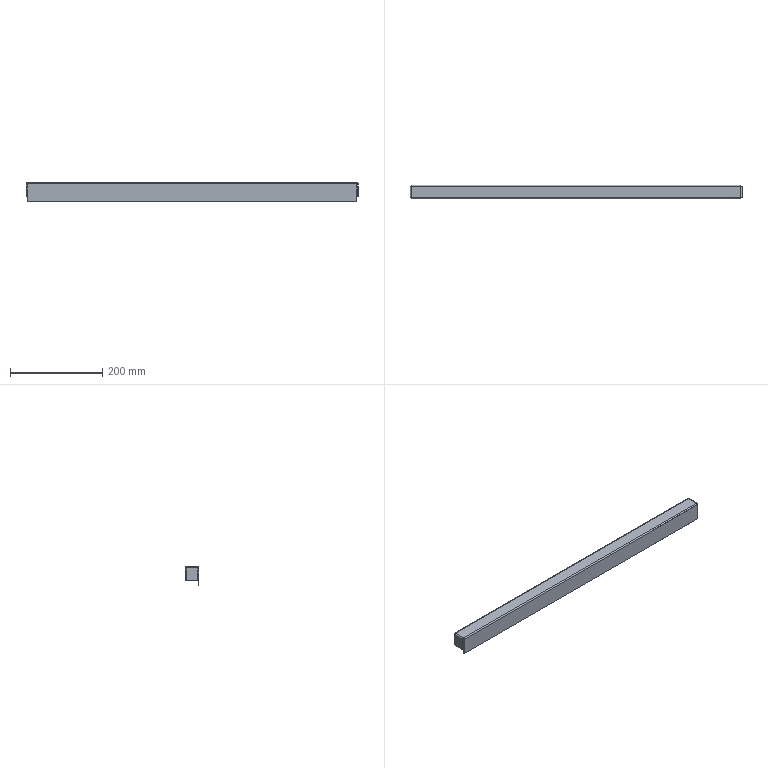Part | STEP file | Front sheet metal baffle | 1 solid | 46 faces | box 720 x 30 x 40 mm | volume 104570 mm3 | plane 22 | cylinder 16 | spline 8 | commonest cylinder face diameters 7 x8 2 x4 5 x4